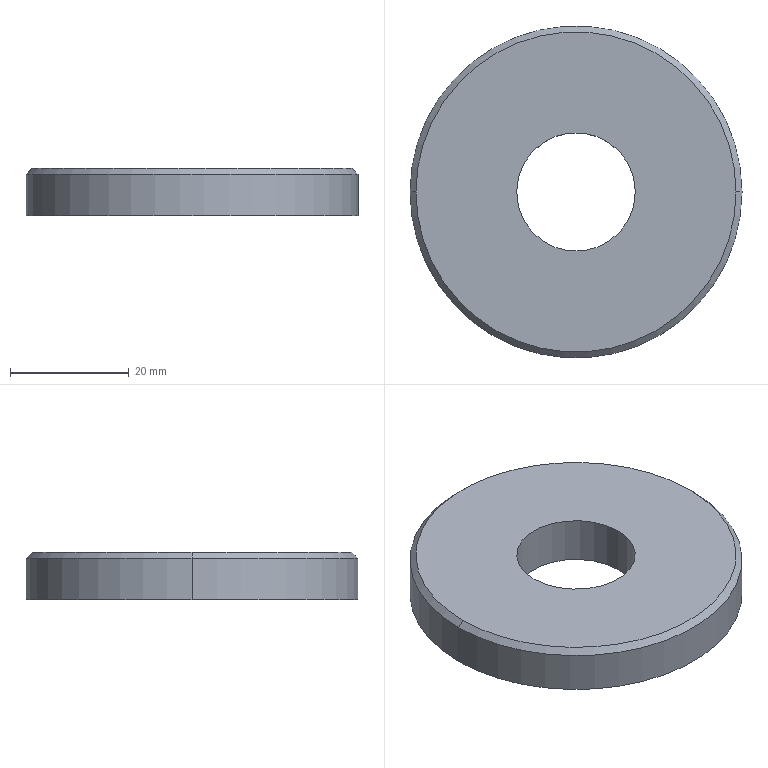Part | STEP file | Cable Carrier Part 3 | 1 solid | 8 faces | box 56 x 56 x 8 mm | volume 17104 mm3 | cylinder 4 | cone 2 | plane 2 | commonest cylinder face diameters 20 x2 56 x2
STEP:
#1=CARTESIAN_POINT('',(0.,0.,0.));
#2=DIRECTION('',(0.,0.,1.));
#3=DIRECTION('',(1.,0.,0.));
#4=AXIS2_PLACEMENT_3D('',#1,#2,#3);
#5=CARTESIAN_POINT('',(27.,0.,8.));
#6=VERTEX_POINT('',#5);
#7=CARTESIAN_POINT('',(-27.,0.,8.));
#8=VERTEX_POINT('',#7);
#9=CARTESIAN_POINT('',(0.,0.,8.));
#10=DIRECTION('',(0.,0.,1.));
#11=DIRECTION('',(1.,0.,0.));
#12=AXIS2_PLACEMENT_3D('',#9,#10,#11);
#13=CIRCLE('',#12,27.);
#14=CARTESIAN_POINT('',(0.,0.,8.));
#15=DIRECTION('',(0.,0.,-1.));
#16=DIRECTION('',(-1.,0.,0.));
#17=AXIS2_PLACEMENT_3D('',#14,#15,#16);
#18=CONICAL_SURFACE('',#17,27.,0.7854);
#19=CARTESIAN_POINT('',(3.142,0.));
#20=DIRECTION('',(-1.,0.));
#21=VECTOR('',#20,1.);
#22=LINE('',#19,#21);
#23=(GEOMETRIC_REPRESENTATION_CONTEXT(2)PARAMETRIC_REPRESENTATION_CONTEXT()REPRESENTATION_CONTEXT('',''));
#24=DEFINITIONAL_REPRESENTATION('',(#22),#23);
#25=PCURVE('',#18,#24);
#26=CARTESIAN_POINT('',(0.,0.,8.));
#27=DIRECTION('',(0.,0.,1.));
#28=DIRECTION('',(1.,0.,0.));
#29=AXIS2_PLACEMENT_3D('',#26,#27,#28);
#30=PLANE('',#29);
#31=CARTESIAN_POINT('',(0.,0.));
#32=DIRECTION('',(1.,0.));
#33=AXIS2_PLACEMENT_2D('',#31,#32);
#34=CIRCLE('',#33,27.);
#35=(GEOMETRIC_REPRESENTATION_CONTEXT(2)PARAMETRIC_REPRESENTATION_CONTEXT()REPRESENTATION_CONTEXT('',''));
#36=DEFINITIONAL_REPRESENTATION('',(#34),#35);
#37=PCURVE('',#30,#36);
#38=SURFACE_CURVE('',#13,(#25,#37),.PCURVE_S1.);
#39=EDGE_CURVE('',#6,#8,#38,.T.);
#40=ORIENTED_EDGE('',*,*,#39,.F.);
#41=CARTESIAN_POINT('',(28.,0.,7.));
#42=VERTEX_POINT('',#41);
#43=CARTESIAN_POINT('',(27.,0.,8.));
#44=DIRECTION('',(0.7071,0.,-0.7071));
#45=VECTOR('',#44,1.);
#46=LINE('',#43,#45);
#47=CARTESIAN_POINT('',(3.142,0.));
#48=DIRECTION('',(0.,1.));
#49=VECTOR('',#48,1.);
#50=LINE('',#47,#49);
#51=(GEOMETRIC_REPRESENTATION_CONTEXT(2)PARAMETRIC_REPRESENTATION_CONTEXT()REPRESENTATION_CONTEXT('',''));
#52=DEFINITIONAL_REPRESENTATION('',(#50),#51);
#53=PCURVE('',#18,#52);
#54=CARTESIAN_POINT('',(0.,0.,8.));
#55=DIRECTION('',(0.,0.,-1.));
#56=DIRECTION('',(-1.,0.,0.));
#57=AXIS2_PLACEMENT_3D('',#54,#55,#56);
#58=CONICAL_SURFACE('',#57,27.,0.7854);
#59=CARTESIAN_POINT('',(3.142,0.));
#60=DIRECTION('',(0.,1.));
#61=VECTOR('',#60,1.);
#62=LINE('',#59,#61);
#63=(GEOMETRIC_REPRESENTATION_CONTEXT(2)PARAMETRIC_REPRESENTATION_CONTEXT()REPRESENTATION_CONTEXT('',''));
#64=DEFINITIONAL_REPRESENTATION('',(#62),#63);
#65=PCURVE('',#58,#64);
#66=SURFACE_CURVE('',#46,(#53,#65),.PCURVE_S1.);
#67=EDGE_CURVE('',#6,#42,#66,.T.);
#68=ORIENTED_EDGE('',*,*,#67,.T.);
#69=CARTESIAN_POINT('',(-28.,0.,7.));
#70=VERTEX_POINT('',#69);
#71=CARTESIAN_POINT('',(0.,0.,7.));
#72=DIRECTION('',(0.,0.,-1.));
#73=DIRECTION('',(1.,0.,0.));
#74=AXIS2_PLACEMENT_3D('',#71,#72,#73);
#75=CIRCLE('',#74,28.);
#76=CARTESIAN_POINT('',(-3.142,1.));
#77=DIRECTION('',(1.,0.));
#78=VECTOR('',#77,1.);
#79=LINE('',#76,#78);
#80=(GEOMETRIC_REPRESENTATION_CONTEXT(2)PARAMETRIC_REPRESENTATION_CONTEXT()REPRESENTATION_CONTEXT('',''));
#81=DEFINITIONAL_REPRESENTATION('',(#79),#80);
#82=PCURVE('',#18,#81);
#83=CARTESIAN_POINT('',(0.,0.,8.));
#84=DIRECTION('',(0.,0.,-1.));
#85=DIRECTION('',(-1.,0.,0.));
#86=AXIS2_PLACEMENT_3D('',#83,#84,#85);
#87=CYLINDRICAL_SURFACE('',#86,28.);
#88=CARTESIAN_POINT('',(-3.142,1.));
#89=DIRECTION('',(1.,0.));
#90=VECTOR('',#89,1.);
#91=LINE('',#88,#90);
#92=(GEOMETRIC_REPRESENTATION_CONTEXT(2)PARAMETRIC_REPRESENTATION_CONTEXT()REPRESENTATION_CONTEXT('',''));
#93=DEFINITIONAL_REPRESENTATION('',(#91),#92);
#94=PCURVE('',#87,#93);
#95=SURFACE_CURVE('',#75,(#82,#94),.PCURVE_S1.);
#96=EDGE_CURVE('',#70,#42,#95,.T.);
#97=ORIENTED_EDGE('',*,*,#96,.F.);
#98=CARTESIAN_POINT('',(-27.,0.,8.));
#99=DIRECTION('',(-0.7071,0.,-0.7071));
#100=VECTOR('',#99,1.);
#101=LINE('',#98,#100);
#102=CARTESIAN_POINT('',(0.,0.));
#103=DIRECTION('',(0.,1.));
#104=VECTOR('',#103,1.);
#105=LINE('',#102,#104);
#106=(GEOMETRIC_REPRESENTATION_CONTEXT(2)PARAMETRIC_REPRESENTATION_CONTEXT()REPRESENTATION_CONTEXT('',''));
#107=DEFINITIONAL_REPRESENTATION('',(#105),#106);
#108=PCURVE('',#18,#107);
#109=CARTESIAN_POINT('',(6.283,0.));
#110=DIRECTION('',(0.,1.));
#111=VECTOR('',#110,1.);
#112=LINE('',#109,#111);
#113=(GEOMETRIC_REPRESENTATION_CONTEXT(2)PARAMETRIC_REPRESENTATION_CONTEXT()REPRESENTATION_CONTEXT('',''));
#114=DEFINITIONAL_REPRESENTATION('',(#112),#113);
#115=PCURVE('',#58,#114);
#116=SURFACE_CURVE('',#101,(#108,#115),.PCURVE_S1.);
#117=EDGE_CURVE('',#8,#70,#116,.T.);
#118=ORIENTED_EDGE('',*,*,#117,.F.);
#119=EDGE_LOOP('',(#40,#68,#97,#118));
#120=FACE_BOUND('',#119,.T.);
#121=ADVANCED_FACE('',(#120),#18,.T.);
#122=CARTESIAN_POINT('',(-10.,0.,8.));
#123=VERTEX_POINT('',#122);
#124=CARTESIAN_POINT('',(-10.,0.,0.));
#125=VERTEX_POINT('',#124);
#126=CARTESIAN_POINT('',(-10.,0.,8.));
#127=DIRECTION('',(0.,0.,-1.));
#128=VECTOR('',#127,1.);
#129=LINE('',#126,#128);
#130=CARTESIAN_POINT('',(0.,0.,8.));
#131=DIRECTION('',(0.,0.,-1.));
#132=DIRECTION('',(-1.,0.,0.));
#133=AXIS2_PLACEMENT_3D('',#130,#131,#132);
#134=CYLINDRICAL_SURFACE('',#133,10.);
#135=CARTESIAN_POINT('',(6.283,0.));
#136=DIRECTION('',(0.,1.));
#137=VECTOR('',#136,1.);
#138=LINE('',#135,#137);
#139=(GEOMETRIC_REPRESENTATION_CONTEXT(2)PARAMETRIC_REPRESENTATION_CONTEXT()REPRESENTATION_CONTEXT('',''));
#140=DEFINITIONAL_REPRESENTATION('',(#138),#139);
#141=PCURVE('',#134,#140);
#142=CARTESIAN_POINT('',(0.,0.,8.));
#143=DIRECTION('',(0.,0.,-1.));
#144=DIRECTION('',(-1.,0.,0.));
#145=AXIS2_PLACEMENT_3D('',#142,#143,#144);
#146=CYLINDRICAL_SURFACE('',#145,10.);
#147=CARTESIAN_POINT('',(0.,0.));
#148=DIRECTION('',(0.,1.));
#149=VECTOR('',#148,1.);
#150=LINE('',#147,#149);
#151=(GEOMETRIC_REPRESENTATION_CONTEXT(2)PARAMETRIC_REPRESENTATION_CONTEXT()REPRESENTATION_CONTEXT('',''));
#152=DEFINITIONAL_REPRESENTATION('',(#150),#151);
#153=PCURVE('',#146,#152);
#154=SURFACE_CURVE('',#129,(#141,#153),.PCURVE_S1.);
#155=EDGE_CURVE('',#123,#125,#154,.T.);
#156=ORIENTED_EDGE('',*,*,#155,.T.);
#157=CARTESIAN_POINT('',(10.,0.,0.));
#158=VERTEX_POINT('',#157);
#159=CARTESIAN_POINT('',(0.,0.,0.));
#160=DIRECTION('',(0.,0.,1.));
#161=DIRECTION('',(1.,0.,0.));
#162=AXIS2_PLACEMENT_3D('',#159,#160,#161);
#163=CIRCLE('',#162,10.);
#164=CARTESIAN_POINT('',(9.425,8.));
#165=DIRECTION('',(-1.,0.));
#166=VECTOR('',#165,1.);
#167=LINE('',#164,#166);
#168=(GEOMETRIC_REPRESENTATION_CONTEXT(2)PARAMETRIC_REPRESENTATION_CONTEXT()REPRESENTATION_CONTEXT('',''));
#169=DEFINITIONAL_REPRESENTATION('',(#167),#168);
#170=PCURVE('',#134,#169);
#171=CARTESIAN_POINT('',(0.,0.,0.));
#172=DIRECTION('',(0.,0.,1.));
#173=DIRECTION('',(1.,0.,0.));
#174=AXIS2_PLACEMENT_3D('',#171,#172,#173);
#175=PLANE('',#174);
#176=CARTESIAN_POINT('',(0.,0.));
#177=DIRECTION('',(1.,0.));
#178=AXIS2_PLACEMENT_2D('',#176,#177);
#179=CIRCLE('',#178,10.);
#180=(GEOMETRIC_REPRESENTATION_CONTEXT(2)PARAMETRIC_REPRESENTATION_CONTEXT()REPRESENTATION_CONTEXT('',''));
#181=DEFINITIONAL_REPRESENTATION('',(#179),#180);
#182=PCURVE('',#175,#181);
#183=SURFACE_CURVE('',#163,(#170,#182),.PCURVE_S1.);
#184=EDGE_CURVE('',#125,#158,#183,.T.);
#185=ORIENTED_EDGE('',*,*,#184,.T.);
#186=CARTESIAN_POINT('',(10.,0.,8.));
#187=VERTEX_POINT('',#186);
#188=CARTESIAN_POINT('',(10.,0.,8.));
#189=DIRECTION('',(0.,0.,-1.));
#190=VECTOR('',#189,1.);
#191=LINE('',#188,#190);
#192=CARTESIAN_POINT('',(3.142,0.));
#193=DIRECTION('',(0.,1.));
#194=VECTOR('',#193,1.);
#195=LINE('',#192,#194);
#196=(GEOMETRIC_REPRESENTATION_CONTEXT(2)PARAMETRIC_REPRESENTATION_CONTEXT()REPRESENTATION_CONTEXT('',''));
#197=DEFINITIONAL_REPRESENTATION('',(#195),#196);
#198=PCURVE('',#134,#197);
#199=CARTESIAN_POINT('',(3.142,0.));
#200=DIRECTION('',(0.,1.));
#201=VECTOR('',#200,1.);
#202=LINE('',#199,#201);
#203=(GEOMETRIC_REPRESENTATION_CONTEXT(2)PARAMETRIC_REPRESENTATION_CONTEXT()REPRESENTATION_CONTEXT('',''));
#204=DEFINITIONAL_REPRESENTATION('',(#202),#203);
#205=PCURVE('',#146,#204);
#206=SURFACE_CURVE('',#191,(#198,#205),.PCURVE_S1.);
#207=EDGE_CURVE('',#187,#158,#206,.T.);
#208=ORIENTED_EDGE('',*,*,#207,.F.);
#209=CARTESIAN_POINT('',(0.,0.,8.));
#210=DIRECTION('',(0.,0.,1.));
#211=DIRECTION('',(1.,0.,0.));
#212=AXIS2_PLACEMENT_3D('',#209,#210,#211);
#213=CIRCLE('',#212,10.);
#214=CARTESIAN_POINT('',(9.425,0.));
#215=DIRECTION('',(-1.,0.));
#216=VECTOR('',#215,1.);
#217=LINE('',#214,#216);
#218=(GEOMETRIC_REPRESENTATION_CONTEXT(2)PARAMETRIC_REPRESENTATION_CONTEXT()REPRESENTATION_CONTEXT('',''));
#219=DEFINITIONAL_REPRESENTATION('',(#217),#218);
#220=PCURVE('',#134,#219);
#221=CARTESIAN_POINT('',(0.,0.));
#222=DIRECTION('',(1.,0.));
#223=AXIS2_PLACEMENT_2D('',#221,#222);
#224=CIRCLE('',#223,10.);
#225=(GEOMETRIC_REPRESENTATION_CONTEXT(2)PARAMETRIC_REPRESENTATION_CONTEXT()REPRESENTATION_CONTEXT('',''));
#226=DEFINITIONAL_REPRESENTATION('',(#224),#225);
#227=PCURVE('',#30,#226);
#228=SURFACE_CURVE('',#213,(#220,#227),.PCURVE_S1.);
#229=EDGE_CURVE('',#123,#187,#228,.T.);
#230=ORIENTED_EDGE('',*,*,#229,.F.);
#231=EDGE_LOOP('',(#156,#185,#208,#230));
#232=FACE_BOUND('',#231,.F.);
#233=ADVANCED_FACE('',(#232),#134,.F.);
#234=ORIENTED_EDGE('',*,*,#96,.T.);
#235=CARTESIAN_POINT('',(28.,0.,0.));
#236=VERTEX_POINT('',#235);
#237=CARTESIAN_POINT('',(28.,0.,8.));
#238=DIRECTION('',(0.,0.,-1.));
#239=VECTOR('',#238,1.);
#240=LINE('',#237,#239);
#241=CARTESIAN_POINT('',(3.142,0.));
#242=DIRECTION('',(0.,1.));
#243=VECTOR('',#242,1.);
#244=LINE('',#241,#243);
#245=(GEOMETRIC_REPRESENTATION_CONTEXT(2)PARAMETRIC_REPRESENTATION_CONTEXT()REPRESENTATION_CONTEXT('',''));
#246=DEFINITIONAL_REPRESENTATION('',(#244),#245);
#247=PCURVE('',#87,#246);
#248=CARTESIAN_POINT('',(0.,0.,8.));
#249=DIRECTION('',(0.,0.,-1.));
#250=DIRECTION('',(-1.,0.,0.));
#251=AXIS2_PLACEMENT_3D('',#248,#249,#250);
#252=CYLINDRICAL_SURFACE('',#251,28.);
#253=CARTESIAN_POINT('',(3.142,0.));
#254=DIRECTION('',(0.,1.));
#255=VECTOR('',#254,1.);
#256=LINE('',#253,#255);
#257=(GEOMETRIC_REPRESENTATION_CONTEXT(2)PARAMETRIC_REPRESENTATION_CONTEXT()REPRESENTATION_CONTEXT('',''));
#258=DEFINITIONAL_REPRESENTATION('',(#256),#257);
#259=PCURVE('',#252,#258);
#260=SURFACE_CURVE('',#240,(#247,#259),.PCURVE_S1.);
#261=EDGE_CURVE('',#42,#236,#260,.T.);
#262=ORIENTED_EDGE('',*,*,#261,.T.);
#263=CARTESIAN_POINT('',(-28.,0.,0.));
#264=VERTEX_POINT('',#263);
#265=CARTESIAN_POINT('',(0.,0.,0.));
#266=DIRECTION('',(0.,0.,1.));
#267=DIRECTION('',(1.,0.,0.));
#268=AXIS2_PLACEMENT_3D('',#265,#266,#267);
#269=CIRCLE('',#268,28.);
#270=CARTESIAN_POINT('',(3.142,8.));
#271=DIRECTION('',(-1.,0.));
#272=VECTOR('',#271,1.);
#273=LINE('',#270,#272);
#274=(GEOMETRIC_REPRESENTATION_CONTEXT(2)PARAMETRIC_REPRESENTATION_CONTEXT()REPRESENTATION_CONTEXT('',''));
#275=DEFINITIONAL_REPRESENTATION('',(#273),#274);
#276=PCURVE('',#87,#275);
#277=CARTESIAN_POINT('',(0.,0.));
#278=DIRECTION('',(1.,0.));
#279=AXIS2_PLACEMENT_2D('',#277,#278);
#280=CIRCLE('',#279,28.);
#281=(GEOMETRIC_REPRESENTATION_CONTEXT(2)PARAMETRIC_REPRESENTATION_CONTEXT()REPRESENTATION_CONTEXT('',''));
#282=DEFINITIONAL_REPRESENTATION('',(#280),#281);
#283=PCURVE('',#175,#282);
#284=SURFACE_CURVE('',#269,(#276,#283),.PCURVE_S1.);
#285=EDGE_CURVE('',#236,#264,#284,.T.);
#286=ORIENTED_EDGE('',*,*,#285,.T.);
#287=CARTESIAN_POINT('',(-28.,0.,8.));
#288=DIRECTION('',(0.,0.,-1.));
#289=VECTOR('',#288,1.);
#290=LINE('',#287,#289);
#291=CARTESIAN_POINT('',(0.,0.));
#292=DIRECTION('',(0.,1.));
#293=VECTOR('',#292,1.);
#294=LINE('',#291,#293);
#295=(GEOMETRIC_REPRESENTATION_CONTEXT(2)PARAMETRIC_REPRESENTATION_CONTEXT()REPRESENTATION_CONTEXT('',''));
#296=DEFINITIONAL_REPRESENTATION('',(#294),#295);
#297=PCURVE('',#87,#296);
#298=CARTESIAN_POINT('',(6.283,0.));
#299=DIRECTION('',(0.,1.));
#300=VECTOR('',#299,1.);
#301=LINE('',#298,#300);
#302=(GEOMETRIC_REPRESENTATION_CONTEXT(2)PARAMETRIC_REPRESENTATION_CONTEXT()REPRESENTATION_CONTEXT('',''));
#303=DEFINITIONAL_REPRESENTATION('',(#301),#302);
#304=PCURVE('',#252,#303);
#305=SURFACE_CURVE('',#290,(#297,#304),.PCURVE_S1.);
#306=EDGE_CURVE('',#70,#264,#305,.T.);
#307=ORIENTED_EDGE('',*,*,#306,.F.);
#308=EDGE_LOOP('',(#234,#262,#286,#307));
#309=FACE_BOUND('',#308,.T.);
#310=ADVANCED_FACE('',(#309),#87,.T.);
#311=CARTESIAN_POINT('',(0.,0.,8.));
#312=DIRECTION('',(0.,0.,1.));
#313=DIRECTION('',(1.,0.,0.));
#314=AXIS2_PLACEMENT_3D('',#311,#312,#313);
#315=CIRCLE('',#314,27.);
#316=CARTESIAN_POINT('',(0.,0.));
#317=DIRECTION('',(1.,0.));
#318=AXIS2_PLACEMENT_2D('',#316,#317);
#319=CIRCLE('',#318,27.);
#320=(GEOMETRIC_REPRESENTATION_CONTEXT(2)PARAMETRIC_REPRESENTATION_CONTEXT()REPRESENTATION_CONTEXT('',''));
#321=DEFINITIONAL_REPRESENTATION('',(#319),#320);
#322=PCURVE('',#30,#321);
#323=CARTESIAN_POINT('',(9.425,0.));
#324=DIRECTION('',(-1.,0.));
#325=VECTOR('',#324,1.);
#326=LINE('',#323,#325);
#327=(GEOMETRIC_REPRESENTATION_CONTEXT(2)PARAMETRIC_REPRESENTATION_CONTEXT()REPRESENTATION_CONTEXT('',''));
#328=DEFINITIONAL_REPRESENTATION('',(#326),#327);
#329=PCURVE('',#58,#328);
#330=SURFACE_CURVE('',#315,(#322,#329),.PCURVE_S1.);
#331=EDGE_CURVE('',#8,#6,#330,.T.);
#332=ORIENTED_EDGE('',*,*,#331,.T.);
#333=ORIENTED_EDGE('',*,*,#39,.T.);
#334=EDGE_LOOP('',(#332,#333));
#335=FACE_BOUND('',#334,.T.);
#336=ORIENTED_EDGE('',*,*,#229,.F.);
#337=CARTESIAN_POINT('',(0.,0.,8.));
#338=DIRECTION('',(0.,0.,1.));
#339=DIRECTION('',(1.,0.,0.));
#340=AXIS2_PLACEMENT_3D('',#337,#338,#339);
#341=CIRCLE('',#340,10.);
#342=CARTESIAN_POINT('',(0.,0.));
#343=DIRECTION('',(1.,0.));
#344=AXIS2_PLACEMENT_2D('',#342,#343);
#345=CIRCLE('',#344,10.);
#346=(GEOMETRIC_REPRESENTATION_CONTEXT(2)PARAMETRIC_REPRESENTATION_CONTEXT()REPRESENTATION_CONTEXT('',''));
#347=DEFINITIONAL_REPRESENTATION('',(#345),#346);
#348=PCURVE('',#30,#347);
#349=CARTESIAN_POINT('',(3.142,0.));
#350=DIRECTION('',(-1.,0.));
#351=VECTOR('',#350,1.);
#352=LINE('',#349,#351);
#353=(GEOMETRIC_REPRESENTATION_CONTEXT(2)PARAMETRIC_REPRESENTATION_CONTEXT()REPRESENTATION_CONTEXT('',''));
#354=DEFINITIONAL_REPRESENTATION('',(#352),#353);
#355=PCURVE('',#146,#354);
#356=SURFACE_CURVE('',#341,(#348,#355),.PCURVE_S1.);
#357=EDGE_CURVE('',#187,#123,#356,.T.);
#358=ORIENTED_EDGE('',*,*,#357,.F.);
#359=EDGE_LOOP('',(#336,#358));
#360=FACE_BOUND('',#359,.T.);
#361=ADVANCED_FACE('',(#335,#360),#30,.T.);
#362=CARTESIAN_POINT('',(0.,0.,0.));
#363=DIRECTION('',(0.,0.,1.));
#364=DIRECTION('',(1.,0.,0.));
#365=AXIS2_PLACEMENT_3D('',#362,#363,#364);
#366=CIRCLE('',#365,28.);
#367=CARTESIAN_POINT('',(0.,0.));
#368=DIRECTION('',(1.,0.));
#369=AXIS2_PLACEMENT_2D('',#367,#368);
#370=CIRCLE('',#369,28.);
#371=(GEOMETRIC_REPRESENTATION_CONTEXT(2)PARAMETRIC_REPRESENTATION_CONTEXT()REPRESENTATION_CONTEXT('',''));
#372=DEFINITIONAL_REPRESENTATION('',(#370),#371);
#373=PCURVE('',#175,#372);
#374=CARTESIAN_POINT('',(9.425,8.));
#375=DIRECTION('',(-1.,0.));
#376=VECTOR('',#375,1.);
#377=LINE('',#374,#376);
#378=(GEOMETRIC_REPRESENTATION_CONTEXT(2)PARAMETRIC_REPRESENTATION_CONTEXT()REPRESENTATION_CONTEXT('',''));
#379=DEFINITIONAL_REPRESENTATION('',(#377),#378);
#380=PCURVE('',#252,#379);
#381=SURFACE_CURVE('',#366,(#373,#380),.PCURVE_S1.);
#382=EDGE_CURVE('',#264,#236,#381,.T.);
#383=ORIENTED_EDGE('',*,*,#382,.F.);
#384=ORIENTED_EDGE('',*,*,#285,.F.);
#385=EDGE_LOOP('',(#383,#384));
#386=FACE_BOUND('',#385,.T.);
#387=ORIENTED_EDGE('',*,*,#184,.T.);
#388=CARTESIAN_POINT('',(0.,0.,0.));
#389=DIRECTION('',(0.,0.,1.));
#390=DIRECTION('',(1.,0.,0.));
#391=AXIS2_PLACEMENT_3D('',#388,#389,#390);
#392=CIRCLE('',#391,10.);
#393=CARTESIAN_POINT('',(0.,0.));
#394=DIRECTION('',(1.,0.));
#395=AXIS2_PLACEMENT_2D('',#393,#394);
#396=CIRCLE('',#395,10.);
#397=(GEOMETRIC_REPRESENTATION_CONTEXT(2)PARAMETRIC_REPRESENTATION_CONTEXT()REPRESENTATION_CONTEXT('',''));
#398=DEFINITIONAL_REPRESENTATION('',(#396),#397);
#399=PCURVE('',#175,#398);
#400=CARTESIAN_POINT('',(3.142,8.));
#401=DIRECTION('',(-1.,0.));
#402=VECTOR('',#401,1.);
#403=LINE('',#400,#402);
#404=(GEOMETRIC_REPRESENTATION_CONTEXT(2)PARAMETRIC_REPRESENTATION_CONTEXT()REPRESENTATION_CONTEXT('',''));
#405=DEFINITIONAL_REPRESENTATION('',(#403),#404);
#406=PCURVE('',#146,#405);
#407=SURFACE_CURVE('',#392,(#399,#406),.PCURVE_S1.);
#408=EDGE_CURVE('',#158,#125,#407,.T.);
#409=ORIENTED_EDGE('',*,*,#408,.T.);
#410=EDGE_LOOP('',(#387,#409));
#411=FACE_BOUND('',#410,.T.);
#412=ADVANCED_FACE('',(#386,#411),#175,.F.);
#413=ORIENTED_EDGE('',*,*,#261,.F.);
#414=CARTESIAN_POINT('',(0.,0.,7.));
#415=DIRECTION('',(0.,0.,-1.));
#416=DIRECTION('',(1.,0.,0.));
#417=AXIS2_PLACEMENT_3D('',#414,#415,#416);
#418=CIRCLE('',#417,28.);
#419=CARTESIAN_POINT('',(3.142,1.));
#420=DIRECTION('',(1.,0.));
#421=VECTOR('',#420,1.);
#422=LINE('',#419,#421);
#423=(GEOMETRIC_REPRESENTATION_CONTEXT(2)PARAMETRIC_REPRESENTATION_CONTEXT()REPRESENTATION_CONTEXT('',''));
#424=DEFINITIONAL_REPRESENTATION('',(#422),#423);
#425=PCURVE('',#252,#424);
#426=CARTESIAN_POINT('',(3.142,1.));
#427=DIRECTION('',(1.,0.));
#428=VECTOR('',#427,1.);
#429=LINE('',#426,#428);
#430=(GEOMETRIC_REPRESENTATION_CONTEXT(2)PARAMETRIC_REPRESENTATION_CONTEXT()REPRESENTATION_CONTEXT('',''));
#431=DEFINITIONAL_REPRESENTATION('',(#429),#430);
#432=PCURVE('',#58,#431);
#433=SURFACE_CURVE('',#418,(#425,#432),.PCURVE_S1.);
#434=EDGE_CURVE('',#42,#70,#433,.T.);
#435=ORIENTED_EDGE('',*,*,#434,.T.);
#436=ORIENTED_EDGE('',*,*,#306,.T.);
#437=ORIENTED_EDGE('',*,*,#382,.T.);
#438=EDGE_LOOP('',(#413,#435,#436,#437));
#439=FACE_BOUND('',#438,.T.);
#440=ADVANCED_FACE('',(#439),#252,.T.);
#441=ORIENTED_EDGE('',*,*,#408,.T.);
#442=ORIENTED_EDGE('',*,*,#155,.F.);
#443=ORIENTED_EDGE('',*,*,#357,.F.);
#444=ORIENTED_EDGE('',*,*,#207,.T.);
#445=EDGE_LOOP('',(#441,#442,#443,#444));
#446=FACE_BOUND('',#445,.F.);
#447=ADVANCED_FACE('',(#446),#146,.F.);
#448=ORIENTED_EDGE('',*,*,#67,.F.);
#449=ORIENTED_EDGE('',*,*,#331,.F.);
#450=ORIENTED_EDGE('',*,*,#117,.T.);
#451=ORIENTED_EDGE('',*,*,#434,.F.);
#452=EDGE_LOOP('',(#448,#449,#450,#451));
#453=FACE_BOUND('',#452,.T.);
#454=ADVANCED_FACE('',(#453),#58,.T.);
#455=CLOSED_SHELL('',(#121,#233,#310,#361,#412,#440,#447,#454));
#456=MANIFOLD_SOLID_BREP('',#455);
#457=(LENGTH_UNIT()NAMED_UNIT(*)SI_UNIT(.MILLI.,.METRE.));
#458=UNCERTAINTY_MEASURE_WITH_UNIT(LENGTH_MEASURE(0.0000001),#457,'','');
#459=(NAMED_UNIT(*)PLANE_ANGLE_UNIT()SI_UNIT($,.RADIAN.));
#460=(NAMED_UNIT(*)SI_UNIT($,.STERADIAN.)SOLID_ANGLE_UNIT());
#461=(GEOMETRIC_REPRESENTATION_CONTEXT(3)GLOBAL_UNCERTAINTY_ASSIGNED_CONTEXT((#458))GLOBAL_UNIT_ASSIGNED_CONTEXT((#457,#459,#460))REPRESENTATION_CONTEXT('',''));
#462=ADVANCED_BREP_SHAPE_REPRESENTATION('',(#4,#456),#461);